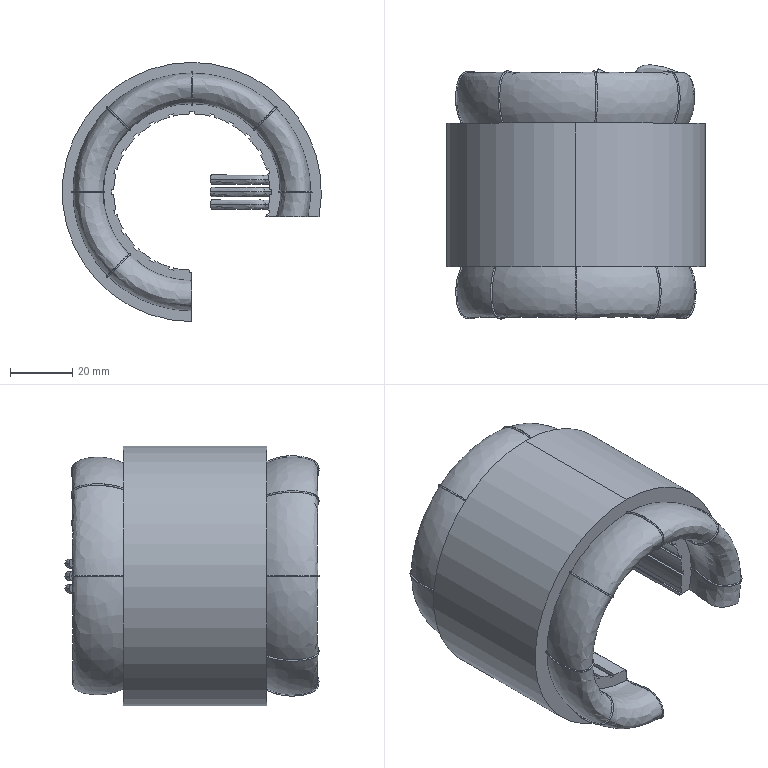Part | STEP file | 1 solid | 139 faces | box 83 x 81.388 x 83 mm | volume 169148 mm3 | plane 80 | spline 37 | cylinder 22 | commonest cylinder face diameters 50 x20 83 x2